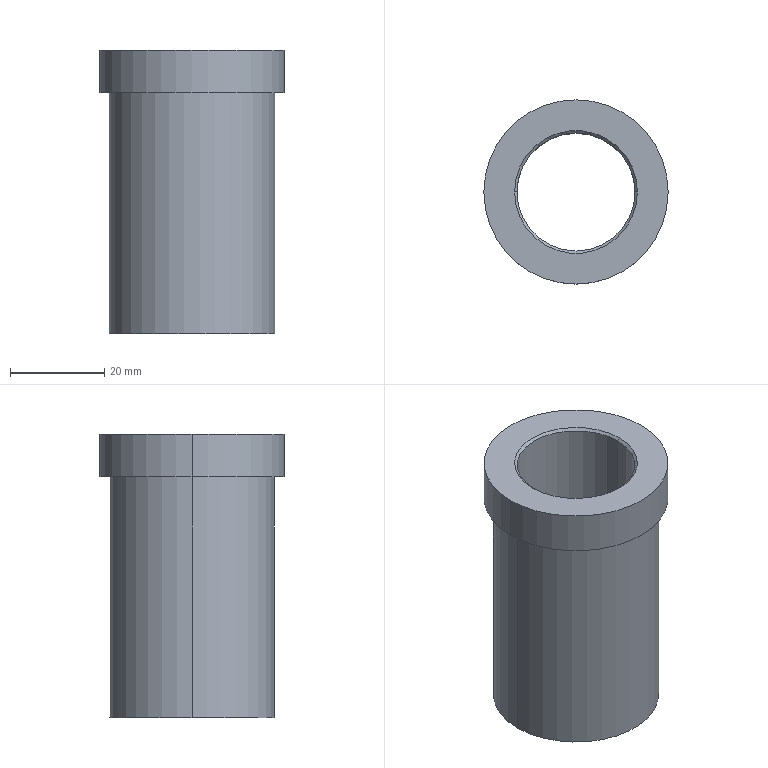Part | SolidWorks | features Revolution 1 | 1 solid | 13 faces | box 39 x 39 x 60 mm | volume 30347 mm3 | cylinder 6 | cone 4 | plane 3 | commonest cylinder face diameters 25 x2 35 x2 39 x2
STEP:
#1=CARTESIAN_POINT('',(-17.5,0.,0.));
#2=VERTEX_POINT('',#1);
#3=CARTESIAN_POINT('',(17.5,0.,0.));
#4=VERTEX_POINT('',#3);
#5=CARTESIAN_POINT('',(0.,0.,0.));
#6=DIRECTION('',(0.,0.,-1.));
#7=DIRECTION('',(-1.,0.,0.));
#8=AXIS2_PLACEMENT_3D('',#5,#6,#7);
#9=CIRCLE('',#8,17.5);
#10=EDGE_CURVE('',#2,#4,#9,.T.);
#11=ORIENTED_EDGE('',*,*,#10,.T.);
#12=CARTESIAN_POINT('',(17.5,0.,-51.));
#13=VERTEX_POINT('',#12);
#14=CARTESIAN_POINT('',(17.5,0.,9.));
#15=DIRECTION('',(0.,0.,-1.));
#16=VECTOR('',#15,1000.);
#17=LINE('',#14,#16);
#18=EDGE_CURVE('',#4,#13,#17,.T.);
#19=ORIENTED_EDGE('',*,*,#18,.T.);
#20=CARTESIAN_POINT('',(-17.5,0.,-51.));
#21=VERTEX_POINT('',#20);
#22=CARTESIAN_POINT('',(0.,0.,-51.));
#23=DIRECTION('',(0.,0.,-1.));
#24=DIRECTION('',(-1.,0.,0.));
#25=AXIS2_PLACEMENT_3D('',#22,#23,#24);
#26=CIRCLE('',#25,17.5);
#27=EDGE_CURVE('',#21,#13,#26,.T.);
#28=ORIENTED_EDGE('',*,*,#27,.F.);
#29=CARTESIAN_POINT('',(-17.5,0.,9.));
#30=DIRECTION('',(0.,0.,-1.));
#31=VECTOR('',#30,1000.);
#32=LINE('',#29,#31);
#33=EDGE_CURVE('',#2,#21,#32,.T.);
#34=ORIENTED_EDGE('',*,*,#33,.F.);
#35=EDGE_LOOP('',(#11,#19,#28,#34));
#36=FACE_OUTER_BOUND('',#35,.T.);
#37=CARTESIAN_POINT('',(0.,0.,9.));
#38=DIRECTION('',(0.,0.,-1.));
#39=DIRECTION('',(-1.,0.,0.));
#40=AXIS2_PLACEMENT_3D('',#37,#38,#39);
#41=CYLINDRICAL_SURFACE('',#40,17.5);
#42=ADVANCED_FACE('',(#36),#41,.T.);
#43=CARTESIAN_POINT('',(12.5,0.,-50.5));
#44=VERTEX_POINT('',#43);
#45=CARTESIAN_POINT('',(-12.5,0.,-50.5));
#46=VERTEX_POINT('',#45);
#47=CARTESIAN_POINT('',(0.,0.,-50.5));
#48=DIRECTION('',(0.,0.,-1.));
#49=DIRECTION('',(-1.,0.,0.));
#50=AXIS2_PLACEMENT_3D('',#47,#48,#49);
#51=CIRCLE('',#50,12.5);
#52=EDGE_CURVE('',#44,#46,#51,.T.);
#53=ORIENTED_EDGE('',*,*,#52,.F.);
#54=CARTESIAN_POINT('',(13.,0.,-51.));
#55=VERTEX_POINT('',#54);
#56=CARTESIAN_POINT('',(12.5,0.,-50.5));
#57=DIRECTION('',(0.7071,0.,-0.7071));
#58=VECTOR('',#57,1000.);
#59=LINE('',#56,#58);
#60=EDGE_CURVE('',#44,#55,#59,.T.);
#61=ORIENTED_EDGE('',*,*,#60,.T.);
#62=CARTESIAN_POINT('',(-13.,0.,-51.));
#63=VERTEX_POINT('',#62);
#64=CARTESIAN_POINT('',(0.,0.,-51.));
#65=DIRECTION('',(0.,0.,-1.));
#66=DIRECTION('',(-1.,0.,0.));
#67=AXIS2_PLACEMENT_3D('',#64,#65,#66);
#68=CIRCLE('',#67,13.);
#69=EDGE_CURVE('',#55,#63,#68,.T.);
#70=ORIENTED_EDGE('',*,*,#69,.T.);
#71=CARTESIAN_POINT('',(-12.5,0.,-50.5));
#72=DIRECTION('',(-0.7071,0.,-0.7071));
#73=VECTOR('',#72,1000.);
#74=LINE('',#71,#73);
#75=EDGE_CURVE('',#46,#63,#74,.T.);
#76=ORIENTED_EDGE('',*,*,#75,.F.);
#77=EDGE_LOOP('',(#53,#61,#70,#76));
#78=FACE_OUTER_BOUND('',#77,.T.);
#79=CARTESIAN_POINT('',(0.,0.,-50.5));
#80=DIRECTION('',(0.,0.,-1.));
#81=DIRECTION('',(-1.,0.,0.));
#82=AXIS2_PLACEMENT_3D('',#79,#80,#81);
#83=CONICAL_SURFACE('',#82,12.5,0.7854);
#84=ADVANCED_FACE('',(#78),#83,.F.);
#85=CARTESIAN_POINT('',(12.5,0.,8.5));
#86=VERTEX_POINT('',#85);
#87=CARTESIAN_POINT('',(-12.5,0.,8.5));
#88=VERTEX_POINT('',#87);
#89=CARTESIAN_POINT('',(0.,0.,8.5));
#90=DIRECTION('',(0.,0.,-1.));
#91=DIRECTION('',(-1.,0.,0.));
#92=AXIS2_PLACEMENT_3D('',#89,#90,#91);
#93=CIRCLE('',#92,12.5);
#94=EDGE_CURVE('',#86,#88,#93,.T.);
#95=ORIENTED_EDGE('',*,*,#94,.F.);
#96=CARTESIAN_POINT('',(12.5,0.,9.));
#97=DIRECTION('',(0.,0.,-1.));
#98=VECTOR('',#97,1000.);
#99=LINE('',#96,#98);
#100=EDGE_CURVE('',#86,#44,#99,.T.);
#101=ORIENTED_EDGE('',*,*,#100,.T.);
#102=ORIENTED_EDGE('',*,*,#52,.T.);
#103=CARTESIAN_POINT('',(-12.5,0.,9.));
#104=DIRECTION('',(0.,0.,-1.));
#105=VECTOR('',#104,1000.);
#106=LINE('',#103,#105);
#107=EDGE_CURVE('',#88,#46,#106,.T.);
#108=ORIENTED_EDGE('',*,*,#107,.F.);
#109=EDGE_LOOP('',(#95,#101,#102,#108));
#110=FACE_OUTER_BOUND('',#109,.T.);
#111=CARTESIAN_POINT('',(0.,0.,9.));
#112=DIRECTION('',(0.,0.,-1.));
#113=DIRECTION('',(-1.,0.,0.));
#114=AXIS2_PLACEMENT_3D('',#111,#112,#113);
#115=CYLINDRICAL_SURFACE('',#114,12.5);
#116=ADVANCED_FACE('',(#110),#115,.F.);
#117=ORIENTED_EDGE('',*,*,#94,.T.);
#118=CARTESIAN_POINT('',(-13.,0.,9.));
#119=VERTEX_POINT('',#118);
#120=CARTESIAN_POINT('',(-13.,0.,9.));
#121=DIRECTION('',(-0.7071,0.,0.7071));
#122=VECTOR('',#121,1000.);
#123=LINE('',#120,#122);
#124=EDGE_CURVE('',#88,#119,#123,.T.);
#125=ORIENTED_EDGE('',*,*,#124,.T.);
#126=CARTESIAN_POINT('',(13.,0.,9.));
#127=VERTEX_POINT('',#126);
#128=CARTESIAN_POINT('',(0.,0.,9.));
#129=DIRECTION('',(0.,0.,-1.));
#130=DIRECTION('',(-1.,0.,0.));
#131=AXIS2_PLACEMENT_3D('',#128,#129,#130);
#132=CIRCLE('',#131,13.);
#133=EDGE_CURVE('',#127,#119,#132,.T.);
#134=ORIENTED_EDGE('',*,*,#133,.F.);
#135=CARTESIAN_POINT('',(13.,0.,9.));
#136=DIRECTION('',(0.7071,0.,0.7071));
#137=VECTOR('',#136,1000.);
#138=LINE('',#135,#137);
#139=EDGE_CURVE('',#86,#127,#138,.T.);
#140=ORIENTED_EDGE('',*,*,#139,.F.);
#141=EDGE_LOOP('',(#117,#125,#134,#140));
#142=FACE_OUTER_BOUND('',#141,.T.);
#143=CARTESIAN_POINT('',(0.,0.,9.));
#144=DIRECTION('',(0.,0.,1.));
#145=DIRECTION('',(1.,0.,0.));
#146=AXIS2_PLACEMENT_3D('',#143,#144,#145);
#147=CONICAL_SURFACE('',#146,13.,0.7854);
#148=ADVANCED_FACE('',(#142),#147,.F.);
#149=CARTESIAN_POINT('',(-19.5,0.,9.));
#150=VERTEX_POINT('',#149);
#151=CARTESIAN_POINT('',(19.5,0.,9.));
#152=VERTEX_POINT('',#151);
#153=CARTESIAN_POINT('',(0.,0.,9.));
#154=DIRECTION('',(0.,0.,-1.));
#155=DIRECTION('',(-1.,0.,0.));
#156=AXIS2_PLACEMENT_3D('',#153,#154,#155);
#157=CIRCLE('',#156,19.5);
#158=EDGE_CURVE('',#150,#152,#157,.T.);
#159=ORIENTED_EDGE('',*,*,#158,.T.);
#160=CARTESIAN_POINT('',(19.5,0.,0.));
#161=VERTEX_POINT('',#160);
#162=CARTESIAN_POINT('',(19.5,0.,9.));
#163=DIRECTION('',(0.,0.,-1.));
#164=VECTOR('',#163,1000.);
#165=LINE('',#162,#164);
#166=EDGE_CURVE('',#152,#161,#165,.T.);
#167=ORIENTED_EDGE('',*,*,#166,.T.);
#168=CARTESIAN_POINT('',(-19.5,0.,0.));
#169=VERTEX_POINT('',#168);
#170=CARTESIAN_POINT('',(0.,0.,0.));
#171=DIRECTION('',(0.,0.,-1.));
#172=DIRECTION('',(-1.,0.,0.));
#173=AXIS2_PLACEMENT_3D('',#170,#171,#172);
#174=CIRCLE('',#173,19.5);
#175=EDGE_CURVE('',#169,#161,#174,.T.);
#176=ORIENTED_EDGE('',*,*,#175,.F.);
#177=CARTESIAN_POINT('',(-19.5,0.,9.));
#178=DIRECTION('',(0.,0.,-1.));
#179=VECTOR('',#178,1000.);
#180=LINE('',#177,#179);
#181=EDGE_CURVE('',#150,#169,#180,.T.);
#182=ORIENTED_EDGE('',*,*,#181,.F.);
#183=EDGE_LOOP('',(#159,#167,#176,#182));
#184=FACE_OUTER_BOUND('',#183,.T.);
#185=CARTESIAN_POINT('',(0.,0.,9.));
#186=DIRECTION('',(0.,0.,-1.));
#187=DIRECTION('',(-1.,0.,0.));
#188=AXIS2_PLACEMENT_3D('',#185,#186,#187);
#189=CYLINDRICAL_SURFACE('',#188,19.5);
#190=ADVANCED_FACE('',(#184),#189,.T.);
#191=ORIENTED_EDGE('',*,*,#175,.T.);
#192=CARTESIAN_POINT('',(0.,0.,0.));
#193=DIRECTION('',(0.,0.,-1.));
#194=DIRECTION('',(-1.,0.,0.));
#195=AXIS2_PLACEMENT_3D('',#192,#193,#194);
#196=CIRCLE('',#195,19.5);
#197=EDGE_CURVE('',#161,#169,#196,.T.);
#198=ORIENTED_EDGE('',*,*,#197,.T.);
#199=EDGE_LOOP('',(#191,#198));
#200=FACE_OUTER_BOUND('',#199,.T.);
#201=ORIENTED_EDGE('',*,*,#10,.F.);
#202=CARTESIAN_POINT('',(0.,0.,0.));
#203=DIRECTION('',(0.,0.,-1.));
#204=DIRECTION('',(-1.,0.,0.));
#205=AXIS2_PLACEMENT_3D('',#202,#203,#204);
#206=CIRCLE('',#205,17.5);
#207=EDGE_CURVE('',#4,#2,#206,.T.);
#208=ORIENTED_EDGE('',*,*,#207,.F.);
#209=EDGE_LOOP('',(#201,#208));
#210=FACE_BOUND('',#209,.T.);
#211=CARTESIAN_POINT('',(17.5,0.,0.));
#212=DIRECTION('',(0.,0.,-1.));
#213=DIRECTION('',(-1.,0.,0.));
#214=AXIS2_PLACEMENT_3D('',#211,#212,#213);
#215=PLANE('',#214);
#216=ADVANCED_FACE('',(#200,#210),#215,.T.);
#217=ORIENTED_EDGE('',*,*,#166,.F.);
#218=CARTESIAN_POINT('',(0.,0.,9.));
#219=DIRECTION('',(0.,0.,-1.));
#220=DIRECTION('',(-1.,0.,0.));
#221=AXIS2_PLACEMENT_3D('',#218,#219,#220);
#222=CIRCLE('',#221,19.5);
#223=EDGE_CURVE('',#152,#150,#222,.T.);
#224=ORIENTED_EDGE('',*,*,#223,.T.);
#225=ORIENTED_EDGE('',*,*,#181,.T.);
#226=ORIENTED_EDGE('',*,*,#197,.F.);
#227=EDGE_LOOP('',(#217,#224,#225,#226));
#228=FACE_OUTER_BOUND('',#227,.T.);
#229=CARTESIAN_POINT('',(0.,0.,9.));
#230=DIRECTION('',(0.,0.,-1.));
#231=DIRECTION('',(-1.,0.,0.));
#232=AXIS2_PLACEMENT_3D('',#229,#230,#231);
#233=CYLINDRICAL_SURFACE('',#232,19.5);
#234=ADVANCED_FACE('',(#228),#233,.T.);
#235=ORIENTED_EDGE('',*,*,#133,.T.);
#236=CARTESIAN_POINT('',(0.,0.,9.));
#237=DIRECTION('',(0.,0.,-1.));
#238=DIRECTION('',(-1.,0.,0.));
#239=AXIS2_PLACEMENT_3D('',#236,#237,#238);
#240=CIRCLE('',#239,13.);
#241=EDGE_CURVE('',#119,#127,#240,.T.);
#242=ORIENTED_EDGE('',*,*,#241,.T.);
#243=EDGE_LOOP('',(#235,#242));
#244=FACE_BOUND('',#243,.T.);
#245=ORIENTED_EDGE('',*,*,#158,.F.);
#246=ORIENTED_EDGE('',*,*,#223,.F.);
#247=EDGE_LOOP('',(#245,#246));
#248=FACE_OUTER_BOUND('',#247,.T.);
#249=CARTESIAN_POINT('',(19.5,0.,9.));
#250=DIRECTION('',(0.,0.,1.));
#251=DIRECTION('',(1.,0.,0.));
#252=AXIS2_PLACEMENT_3D('',#249,#250,#251);
#253=PLANE('',#252);
#254=ADVANCED_FACE('',(#244,#248),#253,.T.);
#255=ORIENTED_EDGE('',*,*,#124,.F.);
#256=CARTESIAN_POINT('',(0.,0.,8.5));
#257=DIRECTION('',(0.,0.,-1.));
#258=DIRECTION('',(-1.,0.,0.));
#259=AXIS2_PLACEMENT_3D('',#256,#257,#258);
#260=CIRCLE('',#259,12.5);
#261=EDGE_CURVE('',#88,#86,#260,.T.);
#262=ORIENTED_EDGE('',*,*,#261,.T.);
#263=ORIENTED_EDGE('',*,*,#139,.T.);
#264=ORIENTED_EDGE('',*,*,#241,.F.);
#265=EDGE_LOOP('',(#255,#262,#263,#264));
#266=FACE_OUTER_BOUND('',#265,.T.);
#267=CARTESIAN_POINT('',(0.,0.,9.));
#268=DIRECTION('',(0.,0.,1.));
#269=DIRECTION('',(1.,0.,0.));
#270=AXIS2_PLACEMENT_3D('',#267,#268,#269);
#271=CONICAL_SURFACE('',#270,13.,0.7854);
#272=ADVANCED_FACE('',(#266),#271,.F.);
#273=ORIENTED_EDGE('',*,*,#100,.F.);
#274=ORIENTED_EDGE('',*,*,#261,.F.);
#275=ORIENTED_EDGE('',*,*,#107,.T.);
#276=CARTESIAN_POINT('',(0.,0.,-50.5));
#277=DIRECTION('',(0.,0.,-1.));
#278=DIRECTION('',(-1.,0.,0.));
#279=AXIS2_PLACEMENT_3D('',#276,#277,#278);
#280=CIRCLE('',#279,12.5);
#281=EDGE_CURVE('',#46,#44,#280,.T.);
#282=ORIENTED_EDGE('',*,*,#281,.T.);
#283=EDGE_LOOP('',(#273,#274,#275,#282));
#284=FACE_OUTER_BOUND('',#283,.T.);
#285=CARTESIAN_POINT('',(0.,0.,9.));
#286=DIRECTION('',(0.,0.,-1.));
#287=DIRECTION('',(-1.,0.,0.));
#288=AXIS2_PLACEMENT_3D('',#285,#286,#287);
#289=CYLINDRICAL_SURFACE('',#288,12.5);
#290=ADVANCED_FACE('',(#284),#289,.F.);
#291=ORIENTED_EDGE('',*,*,#60,.F.);
#292=ORIENTED_EDGE('',*,*,#281,.F.);
#293=ORIENTED_EDGE('',*,*,#75,.T.);
#294=CARTESIAN_POINT('',(0.,0.,-51.));
#295=DIRECTION('',(0.,0.,-1.));
#296=DIRECTION('',(-1.,0.,0.));
#297=AXIS2_PLACEMENT_3D('',#294,#295,#296);
#298=CIRCLE('',#297,13.);
#299=EDGE_CURVE('',#63,#55,#298,.T.);
#300=ORIENTED_EDGE('',*,*,#299,.T.);
#301=EDGE_LOOP('',(#291,#292,#293,#300));
#302=FACE_OUTER_BOUND('',#301,.T.);
#303=CARTESIAN_POINT('',(0.,0.,-50.5));
#304=DIRECTION('',(0.,0.,-1.));
#305=DIRECTION('',(-1.,0.,0.));
#306=AXIS2_PLACEMENT_3D('',#303,#304,#305);
#307=CONICAL_SURFACE('',#306,12.5,0.7854);
#308=ADVANCED_FACE('',(#302),#307,.F.);
#309=ORIENTED_EDGE('',*,*,#27,.T.);
#310=CARTESIAN_POINT('',(0.,0.,-51.));
#311=DIRECTION('',(0.,0.,-1.));
#312=DIRECTION('',(-1.,0.,0.));
#313=AXIS2_PLACEMENT_3D('',#310,#311,#312);
#314=CIRCLE('',#313,17.5);
#315=EDGE_CURVE('',#13,#21,#314,.T.);
#316=ORIENTED_EDGE('',*,*,#315,.T.);
#317=EDGE_LOOP('',(#309,#316));
#318=FACE_OUTER_BOUND('',#317,.T.);
#319=ORIENTED_EDGE('',*,*,#299,.F.);
#320=ORIENTED_EDGE('',*,*,#69,.F.);
#321=EDGE_LOOP('',(#319,#320));
#322=FACE_BOUND('',#321,.T.);
#323=CARTESIAN_POINT('',(13.,0.,-51.));
#324=DIRECTION('',(0.,0.,-1.));
#325=DIRECTION('',(-1.,0.,0.));
#326=AXIS2_PLACEMENT_3D('',#323,#324,#325);
#327=PLANE('',#326);
#328=ADVANCED_FACE('',(#318,#322),#327,.T.);
#329=ORIENTED_EDGE('',*,*,#18,.F.);
#330=ORIENTED_EDGE('',*,*,#207,.T.);
#331=ORIENTED_EDGE('',*,*,#33,.T.);
#332=ORIENTED_EDGE('',*,*,#315,.F.);
#333=EDGE_LOOP('',(#329,#330,#331,#332));
#334=FACE_OUTER_BOUND('',#333,.T.);
#335=CARTESIAN_POINT('',(0.,0.,9.));
#336=DIRECTION('',(0.,0.,-1.));
#337=DIRECTION('',(-1.,0.,0.));
#338=AXIS2_PLACEMENT_3D('',#335,#336,#337);
#339=CYLINDRICAL_SURFACE('',#338,17.5);
#340=ADVANCED_FACE('',(#334),#339,.T.);
#341=CLOSED_SHELL('',(#42,#84,#116,#148,#190,#216,#234,#254,#272,#290,#308,#328,#340));
#342=MANIFOLD_SOLID_BREP('',#341);
#343=CARTESIAN_POINT('',(0.,0.,0.));
#344=DIRECTION('',(0.,0.,1.));
#345=DIRECTION('',(1.,0.,0.));
#346=AXIS2_PLACEMENT_3D('',#343,#344,#345);
#347=(LENGTH_UNIT()NAMED_UNIT(*)SI_UNIT(.MILLI.,.METRE.));
#348=UNCERTAINTY_MEASURE_WITH_UNIT(LENGTH_MEASURE(0.00001),#347,'','');
#349=(NAMED_UNIT(*)PLANE_ANGLE_UNIT()SI_UNIT($,.RADIAN.));
#350=(NAMED_UNIT(*)SI_UNIT($,.STERADIAN.)SOLID_ANGLE_UNIT());
#351=(GEOMETRIC_REPRESENTATION_CONTEXT(3)GLOBAL_UNCERTAINTY_ASSIGNED_CONTEXT((#348))GLOBAL_UNIT_ASSIGNED_CONTEXT((#347,#349,#350))REPRESENTATION_CONTEXT('',''));
#352=ADVANCED_BREP_SHAPE_REPRESENTATION('',(#342,#346),#351);